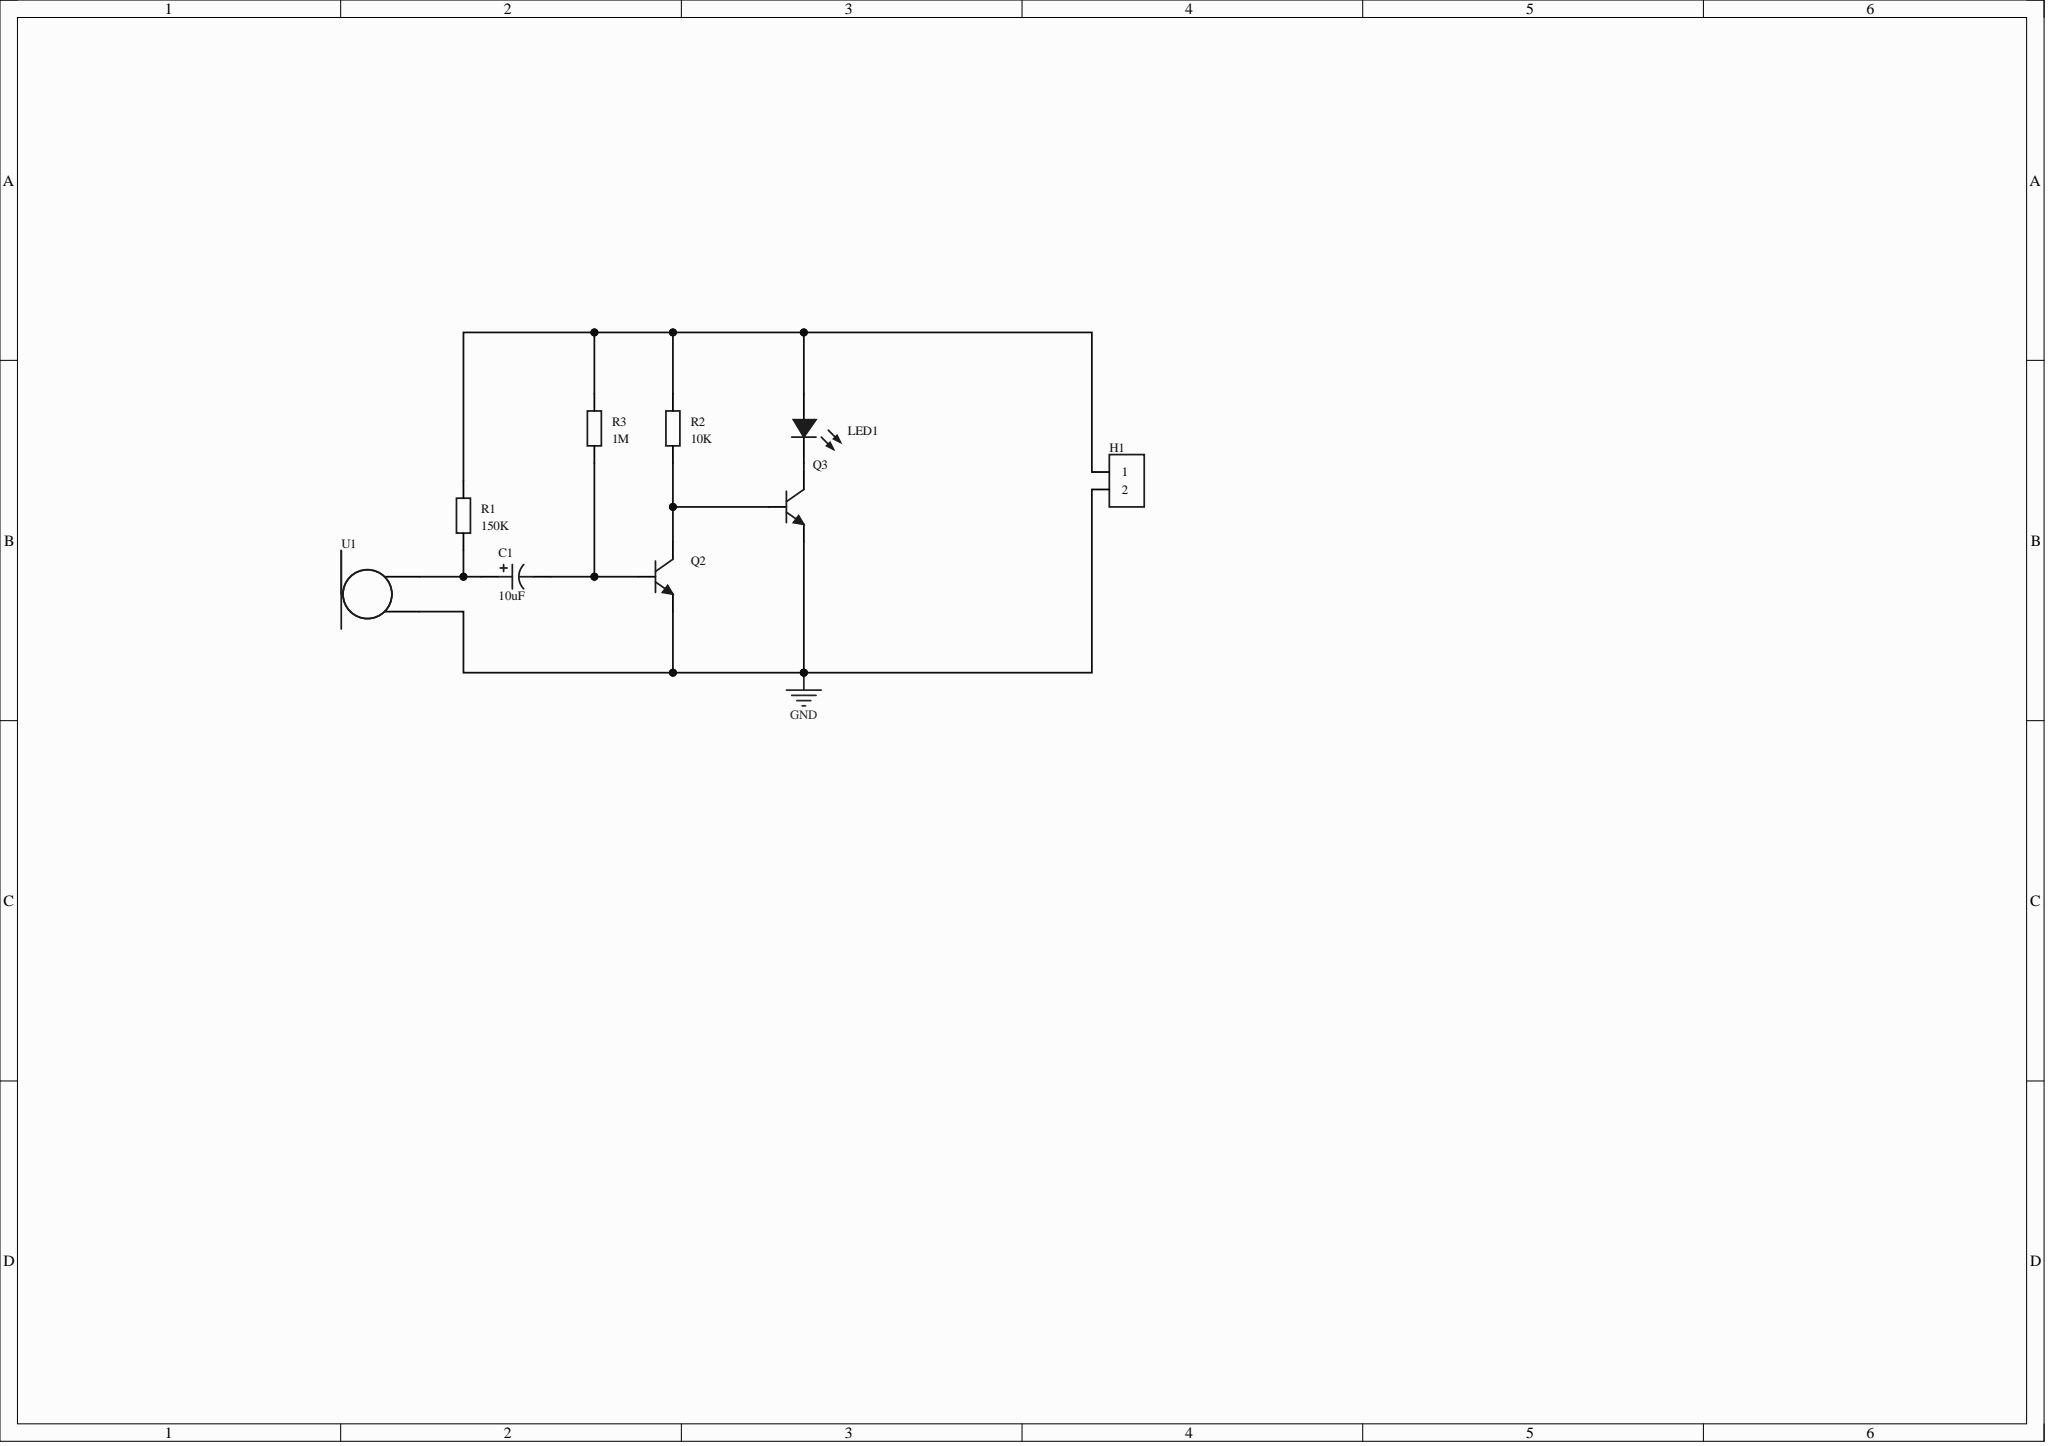Circuit board | Altium Designer | 9 parts | 6 nets
Bill of materials:
Comment,Description,Designator,Footprint,LibRef,Quantity
"10uF","","C1","CAP-TH_BD5.0-P2.00-D0.8-FD-10UF50VC110GL","10UF50VC110GL","1"
"","","H1","HDR-TH_2P-P2.54-V-F","HDR-F_2.54_1x2P","1"
"","","LED1","LED_0603","LED_0603-B","1"
"","","Q2, Q3","S8050_SOT-23","S8050_SOT_NPN","2"
"150K","","R1","R0603","Res_0603","1"
"10K","","R2","R0603","Res_0603","1"
"1M","","R3","R0603","Res_0603","1"
"电流源","","U1","咪头","咪头","1"
Netlist (Protel format):
[
C1
CAP-TH_BD5.0-P2.00-D0.8-FD-10UF50VC110GL
10uF



]
[
H1
HDR-TH_2P-P2.54-V-F




]
[
LED1
LED_0603




]
[
Q2
S8050_SOT-23




]
[
Q3
S8050_SOT-23




]
[
R1
R0603
150K



]
[
R2
R0603
10K



]
[
R3
R0603
1M



]
[
U1
咪头
电流源



]
(
NetQ2_3
Q2-3
Q3-1
R2-1
)
(
NetLED1_1
LED1-1
Q3-3
)
(
NetH1_1
H1-1
LED1-2
R1-2
R2-2
R3-2
)
(
NetC1_2
C1-2
Q2-1
R3-1
)
(
NetC1_1
C1-1
R1-1
U1-2
)
(
GND
H1-2
Q2-2
Q3-2
U1-1
)